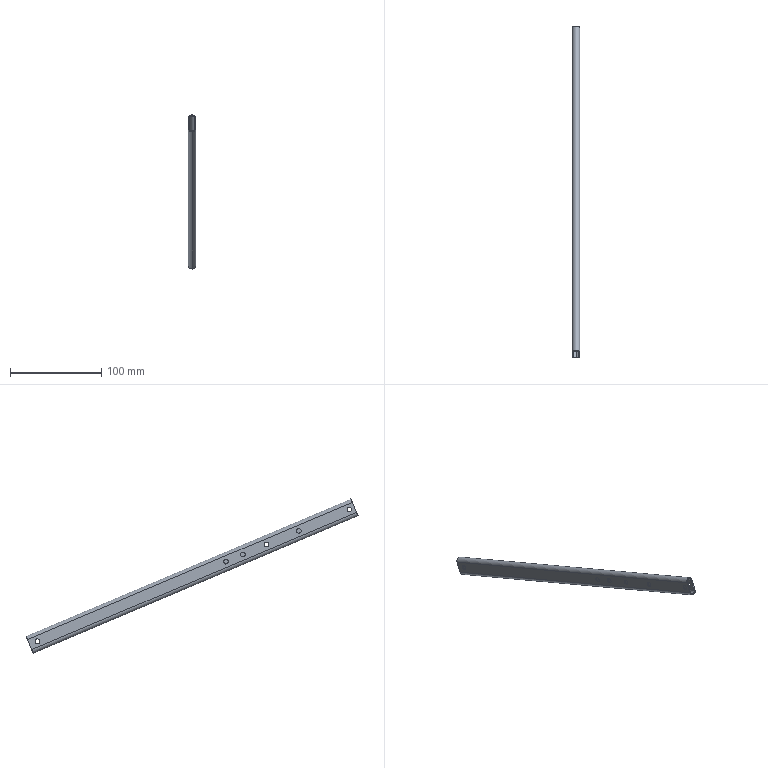Part | SolidWorks | features BaseBody 1 | 1 solid | 30 faces | box 8 x 362.948 x 168.446 mm | volume 20758 mm3 | cylinder 24 | plane 6 | commonest cylinder face diameters 5.2 x18 5.6 x3 8 x3
STEP:
#1=CARTESIAN_POINT('',(170.6,274.633,232.971));
#2=VERTEX_POINT('',#1);
#3=CARTESIAN_POINT('',(170.6,274.633,227.771));
#4=VERTEX_POINT('',#3);
#5=CARTESIAN_POINT('',(170.6,274.633,230.371));
#6=DIRECTION('',(1.,0.,0.));
#7=DIRECTION('',(0.,0.,-1.));
#8=AXIS2_PLACEMENT_3D('',#5,#6,#7);
#9=CIRCLE('',#8,2.6);
#10=EDGE_CURVE('',#2,#4,#9,.T.);
#11=ORIENTED_EDGE('',*,*,#10,.F.);
#12=CARTESIAN_POINT('',(171.8,274.633,232.971));
#13=VERTEX_POINT('',#12);
#14=CARTESIAN_POINT('',(91.8,274.633,232.971));
#15=DIRECTION('',(1.,0.,0.));
#16=VECTOR('',#15,1000.);
#17=LINE('',#14,#16);
#18=EDGE_CURVE('',#2,#13,#17,.T.);
#19=ORIENTED_EDGE('',*,*,#18,.T.);
#20=CARTESIAN_POINT('',(171.8,274.633,227.771));
#21=VERTEX_POINT('',#20);
#22=CARTESIAN_POINT('',(171.8,274.633,230.371));
#23=DIRECTION('',(-1.,0.,0.));
#24=DIRECTION('',(0.,0.,-1.));
#25=AXIS2_PLACEMENT_3D('',#22,#23,#24);
#26=CIRCLE('',#25,2.6);
#27=EDGE_CURVE('',#21,#13,#26,.T.);
#28=ORIENTED_EDGE('',*,*,#27,.F.);
#29=CARTESIAN_POINT('',(91.8,274.633,227.771));
#30=DIRECTION('',(1.,0.,0.));
#31=VECTOR('',#30,1000.);
#32=LINE('',#29,#31);
#33=EDGE_CURVE('',#4,#21,#32,.T.);
#34=ORIENTED_EDGE('',*,*,#33,.F.);
#35=EDGE_LOOP('',(#11,#19,#28,#34));
#36=FACE_OUTER_BOUND('',#35,.T.);
#37=CARTESIAN_POINT('',(91.8,274.633,230.371));
#38=DIRECTION('',(1.,0.,0.));
#39=DIRECTION('',(0.,0.,-1.));
#40=AXIS2_PLACEMENT_3D('',#37,#38,#39);
#41=CYLINDRICAL_SURFACE('',#40,2.6);
#42=ADVANCED_FACE('',(#36),#41,.F.);
#43=CARTESIAN_POINT('',(170.6,365.185,194.722));
#44=VERTEX_POINT('',#43);
#45=CARTESIAN_POINT('',(170.6,365.185,189.522));
#46=VERTEX_POINT('',#45);
#47=CARTESIAN_POINT('',(170.6,365.185,192.122));
#48=DIRECTION('',(1.,0.,0.));
#49=DIRECTION('',(0.,0.,-1.));
#50=AXIS2_PLACEMENT_3D('',#47,#48,#49);
#51=CIRCLE('',#50,2.6);
#52=EDGE_CURVE('',#44,#46,#51,.T.);
#53=ORIENTED_EDGE('',*,*,#52,.F.);
#54=CARTESIAN_POINT('',(171.8,365.185,194.722));
#55=VERTEX_POINT('',#54);
#56=CARTESIAN_POINT('',(91.8,365.185,194.722));
#57=DIRECTION('',(1.,0.,0.));
#58=VECTOR('',#57,1000.);
#59=LINE('',#56,#58);
#60=EDGE_CURVE('',#44,#55,#59,.T.);
#61=ORIENTED_EDGE('',*,*,#60,.T.);
#62=CARTESIAN_POINT('',(171.8,365.185,189.522));
#63=VERTEX_POINT('',#62);
#64=CARTESIAN_POINT('',(171.8,365.185,192.122));
#65=DIRECTION('',(-1.,0.,0.));
#66=DIRECTION('',(0.,0.,-1.));
#67=AXIS2_PLACEMENT_3D('',#64,#65,#66);
#68=CIRCLE('',#67,2.6);
#69=EDGE_CURVE('',#63,#55,#68,.T.);
#70=ORIENTED_EDGE('',*,*,#69,.F.);
#71=CARTESIAN_POINT('',(91.8,365.185,189.522));
#72=DIRECTION('',(1.,0.,0.));
#73=VECTOR('',#72,1000.);
#74=LINE('',#71,#73);
#75=EDGE_CURVE('',#46,#63,#74,.T.);
#76=ORIENTED_EDGE('',*,*,#75,.F.);
#77=EDGE_LOOP('',(#53,#61,#70,#76));
#78=FACE_OUTER_BOUND('',#77,.T.);
#79=CARTESIAN_POINT('',(91.8,365.185,192.122));
#80=DIRECTION('',(1.,0.,0.));
#81=DIRECTION('',(0.,0.,-1.));
#82=AXIS2_PLACEMENT_3D('',#79,#80,#81);
#83=CYLINDRICAL_SURFACE('',#82,2.6);
#84=ADVANCED_FACE('',(#78),#83,.F.);
#85=CARTESIAN_POINT('',(170.6,615.637,88.931));
#86=VERTEX_POINT('',#85);
#87=CARTESIAN_POINT('',(170.6,615.637,83.731));
#88=VERTEX_POINT('',#87);
#89=CARTESIAN_POINT('',(170.6,615.637,86.331));
#90=DIRECTION('',(1.,0.,0.));
#91=DIRECTION('',(0.,0.,-1.));
#92=AXIS2_PLACEMENT_3D('',#89,#90,#91);
#93=CIRCLE('',#92,2.6);
#94=EDGE_CURVE('',#86,#88,#93,.T.);
#95=ORIENTED_EDGE('',*,*,#94,.F.);
#96=CARTESIAN_POINT('',(171.8,615.637,88.931));
#97=VERTEX_POINT('',#96);
#98=CARTESIAN_POINT('',(91.8,615.637,88.931));
#99=DIRECTION('',(1.,0.,0.));
#100=VECTOR('',#99,1000.);
#101=LINE('',#98,#100);
#102=EDGE_CURVE('',#86,#97,#101,.T.);
#103=ORIENTED_EDGE('',*,*,#102,.T.);
#104=CARTESIAN_POINT('',(171.8,615.637,83.731));
#105=VERTEX_POINT('',#104);
#106=CARTESIAN_POINT('',(171.8,615.637,86.331));
#107=DIRECTION('',(-1.,0.,0.));
#108=DIRECTION('',(0.,0.,-1.));
#109=AXIS2_PLACEMENT_3D('',#106,#107,#108);
#110=CIRCLE('',#109,2.6);
#111=EDGE_CURVE('',#105,#97,#110,.T.);
#112=ORIENTED_EDGE('',*,*,#111,.F.);
#113=CARTESIAN_POINT('',(91.8,615.637,83.731));
#114=DIRECTION('',(1.,0.,0.));
#115=VECTOR('',#114,1000.);
#116=LINE('',#113,#115);
#117=EDGE_CURVE('',#88,#105,#116,.T.);
#118=ORIENTED_EDGE('',*,*,#117,.F.);
#119=EDGE_LOOP('',(#95,#103,#112,#118));
#120=FACE_OUTER_BOUND('',#119,.T.);
#121=CARTESIAN_POINT('',(91.8,615.637,86.331));
#122=DIRECTION('',(1.,0.,0.));
#123=DIRECTION('',(0.,0.,-1.));
#124=AXIS2_PLACEMENT_3D('',#121,#122,#123);
#125=CYLINDRICAL_SURFACE('',#124,2.6);
#126=ADVANCED_FACE('',(#120),#125,.F.);
#127=CARTESIAN_POINT('',(163.8,621.916,77.166));
#128=VERTEX_POINT('',#127);
#129=CARTESIAN_POINT('',(167.8,620.36,73.481));
#130=VERTEX_POINT('',#129);
#131=CARTESIAN_POINT('',(167.8,621.916,77.166));
#132=DIRECTION('',(0.,-0.9212,0.3891));
#133=DIRECTION('',(0.,-0.3891,-0.9212));
#134=AXIS2_PLACEMENT_3D('',#131,#132,#133);
#135=CIRCLE('',#134,4.);
#136=EDGE_CURVE('',#128,#130,#135,.T.);
#137=ORIENTED_EDGE('',*,*,#136,.T.);
#138=CARTESIAN_POINT('',(167.8,265.194,223.503));
#139=VERTEX_POINT('',#138);
#140=CARTESIAN_POINT('',(167.8,620.36,73.481));
#141=DIRECTION('',(0.,-0.9212,0.3891));
#142=VECTOR('',#141,1000.);
#143=LINE('',#140,#142);
#144=EDGE_CURVE('',#130,#139,#143,.T.);
#145=ORIENTED_EDGE('',*,*,#144,.T.);
#146=CARTESIAN_POINT('',(163.8,266.75,227.188));
#147=VERTEX_POINT('',#146);
#148=CARTESIAN_POINT('',(167.8,266.75,227.188));
#149=DIRECTION('',(0.,-0.9212,0.3891));
#150=DIRECTION('',(0.,-0.3891,-0.9212));
#151=AXIS2_PLACEMENT_3D('',#148,#149,#150);
#152=CIRCLE('',#151,4.);
#153=EDGE_CURVE('',#147,#139,#152,.T.);
#154=ORIENTED_EDGE('',*,*,#153,.F.);
#155=CARTESIAN_POINT('',(163.8,621.916,77.166));
#156=DIRECTION('',(0.,-0.9212,0.3891));
#157=VECTOR('',#156,1000.);
#158=LINE('',#155,#157);
#159=EDGE_CURVE('',#128,#147,#158,.T.);
#160=ORIENTED_EDGE('',*,*,#159,.F.);
#161=EDGE_LOOP('',(#137,#145,#154,#160));
#162=FACE_OUTER_BOUND('',#161,.T.);
#163=CARTESIAN_POINT('',(167.8,621.916,77.166));
#164=DIRECTION('',(0.,-0.9212,0.3891));
#165=DIRECTION('',(0.,-0.3891,-0.9212));
#166=AXIS2_PLACEMENT_3D('',#163,#164,#165);
#167=CYLINDRICAL_SURFACE('',#166,4.);
#168=ADVANCED_FACE('',(#162),#167,.T.);
#169=CARTESIAN_POINT('',(170.6,621.916,77.166));
#170=VERTEX_POINT('',#169);
#171=CARTESIAN_POINT('',(167.8,620.826,74.586));
#172=VERTEX_POINT('',#171);
#173=CARTESIAN_POINT('',(167.8,621.916,77.166));
#174=DIRECTION('',(0.,0.9212,-0.3891));
#175=DIRECTION('',(0.,-0.3891,-0.9212));
#176=AXIS2_PLACEMENT_3D('',#173,#174,#175);
#177=CIRCLE('',#176,2.8);
#178=EDGE_CURVE('',#170,#172,#177,.T.);
#179=ORIENTED_EDGE('',*,*,#178,.T.);
#180=CARTESIAN_POINT('',(167.8,265.661,224.608));
#181=VERTEX_POINT('',#180);
#182=CARTESIAN_POINT('',(167.8,620.826,74.586));
#183=DIRECTION('',(0.,-0.9212,0.3891));
#184=VECTOR('',#183,1000.);
#185=LINE('',#182,#184);
#186=EDGE_CURVE('',#172,#181,#185,.T.);
#187=ORIENTED_EDGE('',*,*,#186,.T.);
#188=CARTESIAN_POINT('',(170.6,266.75,227.188));
#189=VERTEX_POINT('',#188);
#190=CARTESIAN_POINT('',(167.8,266.75,227.188));
#191=DIRECTION('',(0.,0.9212,-0.3891));
#192=DIRECTION('',(0.,-0.3891,-0.9212));
#193=AXIS2_PLACEMENT_3D('',#190,#191,#192);
#194=CIRCLE('',#193,2.8);
#195=EDGE_CURVE('',#189,#181,#194,.T.);
#196=ORIENTED_EDGE('',*,*,#195,.F.);
#197=CARTESIAN_POINT('',(170.6,621.916,77.166));
#198=DIRECTION('',(0.,-0.9212,0.3891));
#199=VECTOR('',#198,1000.);
#200=LINE('',#197,#199);
#201=EDGE_CURVE('',#170,#189,#200,.T.);
#202=ORIENTED_EDGE('',*,*,#201,.F.);
#203=EDGE_LOOP('',(#179,#187,#196,#202));
#204=FACE_OUTER_BOUND('',#203,.T.);
#205=CARTESIAN_POINT('',(167.8,621.916,77.166));
#206=DIRECTION('',(0.,-0.9212,0.3891));
#207=DIRECTION('',(0.,-0.3891,-0.9212));
#208=AXIS2_PLACEMENT_3D('',#205,#206,#207);
#209=CYLINDRICAL_SURFACE('',#208,2.8);
#210=ADVANCED_FACE('',(#204),#209,.F.);
#211=CARTESIAN_POINT('',(165.,329.905,209.625));
#212=VERTEX_POINT('',#211);
#213=CARTESIAN_POINT('',(165.,329.905,204.425));
#214=VERTEX_POINT('',#213);
#215=CARTESIAN_POINT('',(165.,329.905,207.025));
#216=DIRECTION('',(1.,0.,0.));
#217=DIRECTION('',(0.,0.,1.));
#218=AXIS2_PLACEMENT_3D('',#215,#216,#217);
#219=CIRCLE('',#218,2.6);
#220=EDGE_CURVE('',#212,#214,#219,.T.);
#221=ORIENTED_EDGE('',*,*,#220,.T.);
#222=CARTESIAN_POINT('',(163.8,329.905,204.425));
#223=VERTEX_POINT('',#222);
#224=CARTESIAN_POINT('',(165.8,329.905,204.425));
#225=DIRECTION('',(-1.,0.,0.));
#226=VECTOR('',#225,1000.);
#227=LINE('',#224,#226);
#228=EDGE_CURVE('',#214,#223,#227,.T.);
#229=ORIENTED_EDGE('',*,*,#228,.T.);
#230=CARTESIAN_POINT('',(163.8,329.905,209.625));
#231=VERTEX_POINT('',#230);
#232=CARTESIAN_POINT('',(163.8,329.905,207.025));
#233=DIRECTION('',(1.,0.,0.));
#234=DIRECTION('',(0.,0.,1.));
#235=AXIS2_PLACEMENT_3D('',#232,#233,#234);
#236=CIRCLE('',#235,2.6);
#237=EDGE_CURVE('',#231,#223,#236,.T.);
#238=ORIENTED_EDGE('',*,*,#237,.F.);
#239=CARTESIAN_POINT('',(165.8,329.905,209.625));
#240=DIRECTION('',(-1.,0.,0.));
#241=VECTOR('',#240,1000.);
#242=LINE('',#239,#241);
#243=EDGE_CURVE('',#212,#231,#242,.T.);
#244=ORIENTED_EDGE('',*,*,#243,.F.);
#245=EDGE_LOOP('',(#221,#229,#238,#244));
#246=FACE_OUTER_BOUND('',#245,.T.);
#247=CARTESIAN_POINT('',(165.8,329.905,207.025));
#248=DIRECTION('',(-1.,0.,0.));
#249=DIRECTION('',(0.,0.,1.));
#250=AXIS2_PLACEMENT_3D('',#247,#248,#249);
#251=CYLINDRICAL_SURFACE('',#250,2.6);
#252=ADVANCED_FACE('',(#246),#251,.F.);
#253=CARTESIAN_POINT('',(163.8,274.633,232.971));
#254=VERTEX_POINT('',#253);
#255=CARTESIAN_POINT('',(163.8,274.633,227.771));
#256=VERTEX_POINT('',#255);
#257=CARTESIAN_POINT('',(163.8,274.633,230.371));
#258=DIRECTION('',(1.,0.,0.));
#259=DIRECTION('',(0.,0.,-1.));
#260=AXIS2_PLACEMENT_3D('',#257,#258,#259);
#261=CIRCLE('',#260,2.6);
#262=EDGE_CURVE('',#254,#256,#261,.T.);
#263=ORIENTED_EDGE('',*,*,#262,.F.);
#264=CARTESIAN_POINT('',(165.,274.633,232.971));
#265=VERTEX_POINT('',#264);
#266=CARTESIAN_POINT('',(91.8,274.633,232.971));
#267=DIRECTION('',(1.,0.,0.));
#268=VECTOR('',#267,1000.);
#269=LINE('',#266,#268);
#270=EDGE_CURVE('',#254,#265,#269,.T.);
#271=ORIENTED_EDGE('',*,*,#270,.T.);
#272=CARTESIAN_POINT('',(165.,274.633,227.771));
#273=VERTEX_POINT('',#272);
#274=CARTESIAN_POINT('',(165.,274.633,230.371));
#275=DIRECTION('',(1.,0.,0.));
#276=DIRECTION('',(0.,0.,-1.));
#277=AXIS2_PLACEMENT_3D('',#274,#275,#276);
#278=CIRCLE('',#277,2.6);
#279=EDGE_CURVE('',#265,#273,#278,.T.);
#280=ORIENTED_EDGE('',*,*,#279,.T.);
#281=CARTESIAN_POINT('',(91.8,274.633,227.771));
#282=DIRECTION('',(1.,0.,0.));
#283=VECTOR('',#282,1000.);
#284=LINE('',#281,#283);
#285=EDGE_CURVE('',#256,#273,#284,.T.);
#286=ORIENTED_EDGE('',*,*,#285,.F.);
#287=EDGE_LOOP('',(#263,#271,#280,#286));
#288=FACE_OUTER_BOUND('',#287,.T.);
#289=CARTESIAN_POINT('',(91.8,274.633,230.371));
#290=DIRECTION('',(1.,0.,0.));
#291=DIRECTION('',(0.,0.,-1.));
#292=AXIS2_PLACEMENT_3D('',#289,#290,#291);
#293=CYLINDRICAL_SURFACE('',#292,2.6);
#294=ADVANCED_FACE('',(#288),#293,.F.);
#295=CARTESIAN_POINT('',(163.8,365.185,194.722));
#296=VERTEX_POINT('',#295);
#297=CARTESIAN_POINT('',(163.8,365.185,189.522));
#298=VERTEX_POINT('',#297);
#299=CARTESIAN_POINT('',(163.8,365.185,192.122));
#300=DIRECTION('',(1.,0.,0.));
#301=DIRECTION('',(0.,0.,-1.));
#302=AXIS2_PLACEMENT_3D('',#299,#300,#301);
#303=CIRCLE('',#302,2.6);
#304=EDGE_CURVE('',#296,#298,#303,.T.);
#305=ORIENTED_EDGE('',*,*,#304,.F.);
#306=CARTESIAN_POINT('',(165.,365.185,194.722));
#307=VERTEX_POINT('',#306);
#308=CARTESIAN_POINT('',(91.8,365.185,194.722));
#309=DIRECTION('',(1.,0.,0.));
#310=VECTOR('',#309,1000.);
#311=LINE('',#308,#310);
#312=EDGE_CURVE('',#296,#307,#311,.T.);
#313=ORIENTED_EDGE('',*,*,#312,.T.);
#314=CARTESIAN_POINT('',(165.,365.185,189.522));
#315=VERTEX_POINT('',#314);
#316=CARTESIAN_POINT('',(165.,365.185,192.122));
#317=DIRECTION('',(1.,0.,0.));
#318=DIRECTION('',(0.,0.,-1.));
#319=AXIS2_PLACEMENT_3D('',#316,#317,#318);
#320=CIRCLE('',#319,2.6);
#321=EDGE_CURVE('',#307,#315,#320,.T.);
#322=ORIENTED_EDGE('',*,*,#321,.T.);
#323=CARTESIAN_POINT('',(91.8,365.185,189.522));
#324=DIRECTION('',(1.,0.,0.));
#325=VECTOR('',#324,1000.);
#326=LINE('',#323,#325);
#327=EDGE_CURVE('',#298,#315,#326,.T.);
#328=ORIENTED_EDGE('',*,*,#327,.F.);
#329=EDGE_LOOP('',(#305,#313,#322,#328));
#330=FACE_OUTER_BOUND('',#329,.T.);
#331=CARTESIAN_POINT('',(91.8,365.185,192.122));
#332=DIRECTION('',(1.,0.,0.));
#333=DIRECTION('',(0.,0.,-1.));
#334=AXIS2_PLACEMENT_3D('',#331,#332,#333);
#335=CYLINDRICAL_SURFACE('',#334,2.6);
#336=ADVANCED_FACE('',(#330),#335,.F.);
#337=CARTESIAN_POINT('',(163.8,615.637,88.931));
#338=VERTEX_POINT('',#337);
#339=CARTESIAN_POINT('',(163.8,615.637,83.731));
#340=VERTEX_POINT('',#339);
#341=CARTESIAN_POINT('',(163.8,615.637,86.331));
#342=DIRECTION('',(1.,0.,0.));
#343=DIRECTION('',(0.,0.,-1.));
#344=AXIS2_PLACEMENT_3D('',#341,#342,#343);
#345=CIRCLE('',#344,2.6);
#346=EDGE_CURVE('',#338,#340,#345,.T.);
#347=ORIENTED_EDGE('',*,*,#346,.F.);
#348=CARTESIAN_POINT('',(165.,615.637,88.931));
#349=VERTEX_POINT('',#348);
#350=CARTESIAN_POINT('',(91.8,615.637,88.931));
#351=DIRECTION('',(1.,0.,0.));
#352=VECTOR('',#351,1000.);
#353=LINE('',#350,#352);
#354=EDGE_CURVE('',#338,#349,#353,.T.);
#355=ORIENTED_EDGE('',*,*,#354,.T.);
#356=CARTESIAN_POINT('',(165.,615.637,83.731));
#357=VERTEX_POINT('',#356);
#358=CARTESIAN_POINT('',(165.,615.637,86.331));
#359=DIRECTION('',(1.,0.,0.));
#360=DIRECTION('',(0.,0.,-1.));
#361=AXIS2_PLACEMENT_3D('',#358,#359,#360);
#362=CIRCLE('',#361,2.6);
#363=EDGE_CURVE('',#349,#357,#362,.T.);
#364=ORIENTED_EDGE('',*,*,#363,.T.);
#365=CARTESIAN_POINT('',(91.8,615.637,83.731));
#366=DIRECTION('',(1.,0.,0.));
#367=VECTOR('',#366,1000.);
#368=LINE('',#365,#367);
#369=EDGE_CURVE('',#340,#357,#368,.T.);
#370=ORIENTED_EDGE('',*,*,#369,.F.);
#371=EDGE_LOOP('',(#347,#355,#364,#370));
#372=FACE_OUTER_BOUND('',#371,.T.);
#373=CARTESIAN_POINT('',(91.8,615.637,86.331));
#374=DIRECTION('',(1.,0.,0.));
#375=DIRECTION('',(0.,0.,-1.));
#376=AXIS2_PLACEMENT_3D('',#373,#374,#375);
#377=CYLINDRICAL_SURFACE('',#376,2.6);
#378=ADVANCED_FACE('',(#372),#377,.F.);
#379=CARTESIAN_POINT('',(165.,409.494,176.006));
#380=VERTEX_POINT('',#379);
#381=CARTESIAN_POINT('',(165.,409.494,170.806));
#382=VERTEX_POINT('',#381);
#383=CARTESIAN_POINT('',(165.,409.494,173.406));
#384=DIRECTION('',(1.,0.,0.));
#385=DIRECTION('',(0.,0.,1.));
#386=AXIS2_PLACEMENT_3D('',#383,#384,#385);
#387=CIRCLE('',#386,2.6);
#388=EDGE_CURVE('',#380,#382,#387,.T.);
#389=ORIENTED_EDGE('',*,*,#388,.T.);
#390=CARTESIAN_POINT('',(163.8,409.494,170.806));
#391=VERTEX_POINT('',#390);
#392=CARTESIAN_POINT('',(165.8,409.494,170.806));
#393=DIRECTION('',(-1.,0.,0.));
#394=VECTOR('',#393,1000.);
#395=LINE('',#392,#394);
#396=EDGE_CURVE('',#382,#391,#395,.T.);
#397=ORIENTED_EDGE('',*,*,#396,.T.);
#398=CARTESIAN_POINT('',(163.8,409.494,176.006));
#399=VERTEX_POINT('',#398);
#400=CARTESIAN_POINT('',(163.8,409.494,173.406));
#401=DIRECTION('',(1.,0.,0.));
#402=DIRECTION('',(0.,0.,1.));
#403=AXIS2_PLACEMENT_3D('',#400,#401,#402);
#404=CIRCLE('',#403,2.6);
#405=EDGE_CURVE('',#399,#391,#404,.T.);
#406=ORIENTED_EDGE('',*,*,#405,.F.);
#407=CARTESIAN_POINT('',(165.8,409.494,176.006));
#408=DIRECTION('',(-1.,0.,0.));
#409=VECTOR('',#408,1000.);
#410=LINE('',#407,#409);
#411=EDGE_CURVE('',#380,#399,#410,.T.);
#412=ORIENTED_EDGE('',*,*,#411,.F.);
#413=EDGE_LOOP('',(#389,#397,#406,#412));
#414=FACE_OUTER_BOUND('',#413,.T.);
#415=CARTESIAN_POINT('',(165.8,409.494,173.406));
#416=DIRECTION('',(-1.,0.,0.));
#417=DIRECTION('',(0.,0.,1.));
#418=AXIS2_PLACEMENT_3D('',#415,#416,#417);
#419=CYLINDRICAL_SURFACE('',#418,2.6);
#420=ADVANCED_FACE('',(#414),#419,.F.);
#421=CARTESIAN_POINT('',(165.,391.07,183.788));
#422=VERTEX_POINT('',#421);
#423=CARTESIAN_POINT('',(165.,391.07,178.588));
#424=VERTEX_POINT('',#423);
#425=CARTESIAN_POINT('',(165.,391.07,181.188));
#426=DIRECTION('',(1.,0.,0.));
#427=DIRECTION('',(0.,0.,1.));
#428=AXIS2_PLACEMENT_3D('',#425,#426,#427);
#429=CIRCLE('',#428,2.6);
#430=EDGE_CURVE('',#422,#424,#429,.T.);
#431=ORIENTED_EDGE('',*,*,#430,.T.);
#432=CARTESIAN_POINT('',(163.8,391.07,178.588));
#433=VERTEX_POINT('',#432);
#434=CARTESIAN_POINT('',(165.8,391.07,178.588));
#435=DIRECTION('',(-1.,0.,0.));
#436=VECTOR('',#435,1000.);
#437=LINE('',#434,#436);
#438=EDGE_CURVE('',#424,#433,#437,.T.);
#439=ORIENTED_EDGE('',*,*,#438,.T.);
#440=CARTESIAN_POINT('',(163.8,391.07,183.788));
#441=VERTEX_POINT('',#440);
#442=CARTESIAN_POINT('',(163.8,391.07,181.188));
#443=DIRECTION('',(1.,0.,0.));
#444=DIRECTION('',(0.,0.,1.));
#445=AXIS2_PLACEMENT_3D('',#442,#443,#444);
#446=CIRCLE('',#445,2.6);
#447=EDGE_CURVE('',#441,#433,#446,.T.);
#448=ORIENTED_EDGE('',*,*,#447,.F.);
#449=CARTESIAN_POINT('',(165.8,391.07,183.788));
#450=DIRECTION('',(-1.,0.,0.));
#451=VECTOR('',#450,1000.);
#452=LINE('',#449,#451);
#453=EDGE_CURVE('',#422,#441,#452,.T.);
#454=ORIENTED_EDGE('',*,*,#453,.F.);
#455=EDGE_LOOP('',(#431,#439,#448,#454));
#456=FACE_OUTER_BOUND('',#455,.T.);
#457=CARTESIAN_POINT('',(165.8,391.07,181.188));
#458=DIRECTION('',(-1.,0.,0.));
#459=DIRECTION('',(0.,0.,1.));
#460=AXIS2_PLACEMENT_3D('',#457,#458,#459);
#461=CYLINDRICAL_SURFACE('',#460,2.6);
#462=ADVANCED_FACE('',(#456),#461,.F.);
#463=CARTESIAN_POINT('',(163.8,271.419,238.242));
#464=VERTEX_POINT('',#463);
#465=CARTESIAN_POINT('',(171.8,271.419,238.242));
#466=VERTEX_POINT('',#465);
#467=CARTESIAN_POINT('',(167.8,271.419,238.242));
#468=DIRECTION('',(0.,0.9212,-0.3891));
#469=DIRECTION('',(0.,-0.3891,-0.9212));
#470=AXIS2_PLACEMENT_3D('',#467,#468,#469);
#471=CIRCLE('',#470,4.);
#472=EDGE_CURVE('',#464,#466,#471,.T.);
#473=ORIENTED_EDGE('',*,*,#472,.T.);
#474=CARTESIAN_POINT('',(171.8,626.585,88.22));
#475=VERTEX_POINT('',#474);
#476=CARTESIAN_POINT('',(171.8,626.585,88.22));
#477=DIRECTION('',(0.,0.9212,-0.3891));
#478=VECTOR('',#477,1000.);
#479=LINE('',#476,#478);
#480=EDGE_CURVE('',#466,#475,#479,.T.);
#481=ORIENTED_EDGE('',*,*,#480,.T.);
#482=CARTESIAN_POINT('',(163.8,626.585,88.22));
#483=VERTEX_POINT('',#482);
#484=CARTESIAN_POINT('',(167.8,626.585,88.22));
#485=DIRECTION('',(0.,-0.9212,0.3891));
#486=DIRECTION('',(0.,-0.3891,-0.9212));
#487=AXIS2_PLACEMENT_3D('',#484,#485,#486);
#488=CIRCLE('',#487,4.);
#489=EDGE_CURVE('',#475,#483,#488,.T.);
#490=ORIENTED_EDGE('',*,*,#489,.T.);
#491=CARTESIAN_POINT('',(163.8,626.585,88.22));
#492=DIRECTION('',(0.,-0.9212,0.3891));
#493=VECTOR('',#492,1000.);
#494=LINE('',#491,#493);
#495=EDGE_CURVE('',#483,#464,#494,.T.);
#496=ORIENTED_EDGE('',*,*,#495,.T.);
#497=EDGE_LOOP('',(#473,#481,#490,#496));
#498=FACE_OUTER_BOUND('',#497,.T.);
#499=CARTESIAN_POINT('',(167.8,626.585,88.22));
#500=DIRECTION('',(0.,-0.9212,0.3891));
#501=DIRECTION('',(0.,-0.3891,-0.9212));
#502=AXIS2_PLACEMENT_3D('',#499,#500,#501);
#503=CYLINDRICAL_SURFACE('',#502,4.);
#504=ADVANCED_FACE('',(#498),#503,.T.);
#505=ORIENTED_EDGE('',*,*,#27,.T.);
#506=CARTESIAN_POINT('',(171.8,274.633,230.371));
#507=DIRECTION('',(-1.,0.,0.));
#508=DIRECTION('',(0.,0.,-1.));
#509=AXIS2_PLACEMENT_3D('',#506,#507,#508);
#510=CIRCLE('',#509,2.6);
#511=EDGE_CURVE('',#13,#21,#510,.T.);
#512=ORIENTED_EDGE('',*,*,#511,.T.);
#513=EDGE_LOOP('',(#505,#512));
#514=FACE_BOUND('',#513,.T.);
#515=ORIENTED_EDGE('',*,*,#69,.T.);
#516=CARTESIAN_POINT('',(171.8,365.185,192.122));
#517=DIRECTION('',(-1.,0.,0.));
#518=DIRECTION('',(0.,0.,-1.));
#519=AXIS2_PLACEMENT_3D('',#516,#517,#518);
#520=CIRCLE('',#519,2.6);
#521=EDGE_CURVE('',#55,#63,#520,.T.);
#522=ORIENTED_EDGE('',*,*,#521,.T.);
#523=EDGE_LOOP('',(#515,#522));
#524=FACE_BOUND('',#523,.T.);
#525=ORIENTED_EDGE('',*,*,#111,.T.);
#526=CARTESIAN_POINT('',(171.8,615.637,86.331));
#527=DIRECTION('',(-1.,0.,0.));
#528=DIRECTION('',(0.,0.,-1.));
#529=AXIS2_PLACEMENT_3D('',#526,#527,#528);
#530=CIRCLE('',#529,2.6);
#531=EDGE_CURVE('',#97,#105,#530,.T.);
#532=ORIENTED_EDGE('',*,*,#531,.T.);
#533=EDGE_LOOP('',(#525,#532));
#534=FACE_BOUND('',#533,.T.);
#535=CARTESIAN_POINT('',(171.8,266.75,227.188));
#536=VERTEX_POINT('',#535);
#537=CARTESIAN_POINT('',(171.8,271.419,238.242));
#538=DIRECTION('',(0.,-0.3891,-0.9212));
#539=VECTOR('',#538,1000.);
#540=LINE('',#537,#539);
#541=EDGE_CURVE('',#466,#536,#540,.T.);
#542=ORIENTED_EDGE('',*,*,#541,.T.);
#543=CARTESIAN_POINT('',(171.8,621.916,77.166));
#544=VERTEX_POINT('',#543);
#545=CARTESIAN_POINT('',(171.8,266.75,227.188));
#546=DIRECTION('',(0.,0.9212,-0.3891));
#547=VECTOR('',#546,1000.);
#548=LINE('',#545,#547);
#549=EDGE_CURVE('',#536,#544,#548,.T.);
#550=ORIENTED_EDGE('',*,*,#549,.T.);
#551=CARTESIAN_POINT('',(171.8,621.916,77.166));
#552=DIRECTION('',(0.,0.3891,0.9212));
#553=VECTOR('',#552,1000.);
#554=LINE('',#551,#553);
#555=EDGE_CURVE('',#544,#475,#554,.T.);
#556=ORIENTED_EDGE('',*,*,#555,.T.);
#557=ORIENTED_EDGE('',*,*,#480,.F.);
#558=EDGE_LOOP('',(#542,#550,#556,#557));
#559=FACE_OUTER_BOUND('',#558,.T.);
#560=CARTESIAN_POINT('',(171.8,621.916,77.166));
#561=DIRECTION('',(1.,0.,0.));
#562=DIRECTION('',(0.,0.,-1.));
#563=AXIS2_PLACEMENT_3D('',#560,#561,#562);
#564=PLANE('',#563);
#565=ADVANCED_FACE('',(#514,#524,#534,#559),#564,.T.);
#566=CARTESIAN_POINT('',(165.,266.75,227.188));
#567=VERTEX_POINT('',#566);
#568=CARTESIAN_POINT('',(165.,271.419,238.242));
#569=VERTEX_POINT('',#568);
#570=CARTESIAN_POINT('',(165.,266.75,227.188));
#571=DIRECTION('',(0.,0.3891,0.9212));
#572=VECTOR('',#571,1000.);
#573=LINE('',#570,#572);
#574=EDGE_CURVE('',#567,#569,#573,.T.);
#575=ORIENTED_EDGE('',*,*,#574,.T.);
#576=CARTESIAN_POINT('',(170.6,271.419,238.242));
#577=VERTEX_POINT('',#576);
#578=CARTESIAN_POINT('',(167.8,271.419,238.242));
#579=DIRECTION('',(0.,0.9212,-0.3891));
#580=DIRECTION('',(0.,-0.3891,-0.9212));
#581=AXIS2_PLACEMENT_3D('',#578,#579,#580);
#582=CIRCLE('',#581,2.8);
#583=EDGE_CURVE('',#569,#577,#582,.T.);
#584=ORIENTED_EDGE('',*,*,#583,.T.);
#585=CARTESIAN_POINT('',(170.6,266.75,227.188));
#586=DIRECTION('',(0.,-0.3891,-0.9212));
#587=VECTOR('',#586,1000.);
#588=LINE('',#585,#587);
#589=EDGE_CURVE('',#577,#189,#588,.T.);
#590=ORIENTED_EDGE('',*,*,#589,.T.);
#591=ORIENTED_EDGE('',*,*,#195,.T.);
#592=CARTESIAN_POINT('',(167.8,266.75,227.188));
#593=DIRECTION('',(0.,0.9212,-0.3891));
#594=DIRECTION('',(0.,-0.3891,-0.9212));
#595=AXIS2_PLACEMENT_3D('',#592,#593,#594);
#596=CIRCLE('',#595,2.8);
#597=EDGE_CURVE('',#181,#567,#596,.T.);
#598=ORIENTED_EDGE('',*,*,#597,.T.);
#599=EDGE_LOOP('',(#575,#584,#590,#591,#598));
#600=FACE_BOUND('',#599,.T.);
#601=ORIENTED_EDGE('',*,*,#153,.T.);
#602=CARTESIAN_POINT('',(167.8,266.75,227.188));
#603=DIRECTION('',(0.,-0.9212,0.3891));
#604=DIRECTION('',(0.,-0.3891,-0.9212));
#605=AXIS2_PLACEMENT_3D('',#602,#603,#604);
#606=CIRCLE('',#605,4.);
#607=EDGE_CURVE('',#139,#536,#606,.T.);
#608=ORIENTED_EDGE('',*,*,#607,.T.);
#609=ORIENTED_EDGE('',*,*,#541,.F.);
#610=ORIENTED_EDGE('',*,*,#472,.F.);
#611=CARTESIAN_POINT('',(163.8,266.75,227.188));
#612=DIRECTION('',(0.,-0.3891,-0.9212));
#613=VECTOR('',#612,1000.);
#614=LINE('',#611,#613);
#615=EDGE_CURVE('',#464,#147,#614,.T.);
#616=ORIENTED_EDGE('',*,*,#615,.T.);
#617=EDGE_LOOP('',(#601,#608,#609,#610,#616));
#618=FACE_OUTER_BOUND('',#617,.T.);
#619=CARTESIAN_POINT('',(167.8,266.75,227.188));
#620=DIRECTION('',(0.,-0.9212,0.3891));
#621=DIRECTION('',(0.,-0.3891,-0.9212));
#622=AXIS2_PLACEMENT_3D('',#619,#620,#621);
#623=PLANE('',#622);
#624=ADVANCED_FACE('',(#600,#618),#623,.T.);
#625=ORIENTED_EDGE('',*,*,#237,.T.);
#626=CARTESIAN_POINT('',(163.8,329.905,207.025));
#627=DIRECTION('',(1.,0.,0.));
#628=DIRECTION('',(0.,0.,1.));
#629=AXIS2_PLACEMENT_3D('',#626,#627,#628);
#630=CIRCLE('',#629,2.6);
#631=EDGE_CURVE('',#223,#231,#630,.T.);
#632=ORIENTED_EDGE('',*,*,#631,.T.);
#633=EDGE_LOOP('',(#625,#632));
#634=FACE_BOUND('',#633,.T.);
#635=CARTESIAN_POINT('',(163.8,274.633,230.371));
#636=DIRECTION('',(1.,0.,0.));
#637=DIRECTION('',(0.,0.,-1.));
#638=AXIS2_PLACEMENT_3D('',#635,#636,#637);
#639=CIRCLE('',#638,2.6);
#640=EDGE_CURVE('',#256,#254,#639,.T.);
#641=ORIENTED_EDGE('',*,*,#640,.T.);
#642=ORIENTED_EDGE('',*,*,#262,.T.);
#643=EDGE_LOOP('',(#641,#642));
#644=FACE_BOUND('',#643,.T.);
#645=CARTESIAN_POINT('',(163.8,365.185,192.122));
#646=DIRECTION('',(1.,0.,0.));
#647=DIRECTION('',(0.,0.,-1.));
#648=AXIS2_PLACEMENT_3D('',#645,#646,#647);
#649=CIRCLE('',#648,2.6);
#650=EDGE_CURVE('',#298,#296,#649,.T.);
#651=ORIENTED_EDGE('',*,*,#650,.T.);
#652=ORIENTED_EDGE('',*,*,#304,.T.);
#653=EDGE_LOOP('',(#651,#652));
#654=FACE_BOUND('',#653,.T.);
#655=CARTESIAN_POINT('',(163.8,615.637,86.331));
#656=DIRECTION('',(1.,0.,0.));
#657=DIRECTION('',(0.,0.,-1.));
#658=AXIS2_PLACEMENT_3D('',#655,#656,#657);
#659=CIRCLE('',#658,2.6);
#660=EDGE_CURVE('',#340,#338,#659,.T.);
#661=ORIENTED_EDGE('',*,*,#660,.T.);
#662=ORIENTED_EDGE('',*,*,#346,.T.);
#663=EDGE_LOOP('',(#661,#662));
#664=FACE_BOUND('',#663,.T.);
#665=ORIENTED_EDGE('',*,*,#615,.F.);
#666=ORIENTED_EDGE('',*,*,#495,.F.);
#667=CARTESIAN_POINT('',(163.8,626.585,88.22));
#668=DIRECTION('',(0.,-0.3891,-0.9212));
#669=VECTOR('',#668,1000.);
#670=LINE('',#667,#669);
#671=EDGE_CURVE('',#483,#128,#670,.T.);
#672=ORIENTED_EDGE('',*,*,#671,.T.);
#673=ORIENTED_EDGE('',*,*,#159,.T.);
#674=EDGE_LOOP('',(#665,#666,#672,#673));
#675=FACE_OUTER_BOUND('',#674,.T.);
#676=ORIENTED_EDGE('',*,*,#405,.T.);
#677=CARTESIAN_POINT('',(163.8,409.494,173.406));
#678=DIRECTION('',(1.,0.,0.));
#679=DIRECTION('',(0.,0.,1.));
#680=AXIS2_PLACEMENT_3D('',#677,#678,#679);
#681=CIRCLE('',#680,2.6);
#682=EDGE_CURVE('',#391,#399,#681,.T.);
#683=ORIENTED_EDGE('',*,*,#682,.T.);
#684=EDGE_LOOP('',(#676,#683));
#685=FACE_BOUND('',#684,.T.);
#686=ORIENTED_EDGE('',*,*,#447,.T.);
#687=CARTESIAN_POINT('',(163.8,391.07,181.188));
#688=DIRECTION('',(1.,0.,0.));
#689=DIRECTION('',(0.,0.,1.));
#690=AXIS2_PLACEMENT_3D('',#687,#688,#689);
#691=CIRCLE('',#690,2.6);
#692=EDGE_CURVE('',#433,#441,#691,.T.);
#693=ORIENTED_EDGE('',*,*,#692,.T.);
#694=EDGE_LOOP('',(#686,#693));
#695=FACE_BOUND('',#694,.T.);
#696=CARTESIAN_POINT('',(163.8,621.916,77.166));
#697=DIRECTION('',(-1.,0.,0.));
#698=DIRECTION('',(0.,0.,1.));
#699=AXIS2_PLACEMENT_3D('',#696,#697,#698);
#700=PLANE('',#699);
#701=ADVANCED_FACE('',(#634,#644,#654,#664,#675,#685,#695),#700,.T.);
#702=CARTESIAN_POINT('',(170.6,626.585,88.22));
#703=VERTEX_POINT('',#702);
#704=CARTESIAN_POINT('',(170.6,621.916,77.166));
#705=DIRECTION('',(0.,-0.3891,-0.9212));
#706=VECTOR('',#705,1000.);
#707=LINE('',#704,#706);
#708=EDGE_CURVE('',#703,#170,#707,.T.);
#709=ORIENTED_EDGE('',*,*,#708,.F.);
#710=CARTESIAN_POINT('',(165.,626.585,88.22));
#711=VERTEX_POINT('',#710);
#712=CARTESIAN_POINT('',(167.8,626.585,88.22));
#713=DIRECTION('',(0.,0.9212,-0.3891));
#714=DIRECTION('',(0.,-0.3891,-0.9212));
#715=AXIS2_PLACEMENT_3D('',#712,#713,#714);
#716=CIRCLE('',#715,2.8);
#717=EDGE_CURVE('',#711,#703,#716,.T.);
#718=ORIENTED_EDGE('',*,*,#717,.F.);
#719=CARTESIAN_POINT('',(165.,621.916,77.166));
#720=VERTEX_POINT('',#719);
#721=CARTESIAN_POINT('',(165.,621.916,77.166));
#722=DIRECTION('',(0.,0.3891,0.9212));
#723=VECTOR('',#722,1000.);
#724=LINE('',#721,#723);
#725=EDGE_CURVE('',#720,#711,#724,.T.);
#726=ORIENTED_EDGE('',*,*,#725,.F.);
#727=CARTESIAN_POINT('',(167.8,621.916,77.166));
#728=DIRECTION('',(0.,0.9212,-0.3891));
#729=DIRECTION('',(0.,-0.3891,-0.9212));
#730=AXIS2_PLACEMENT_3D('',#727,#728,#729);
#731=CIRCLE('',#730,2.8);
#732=EDGE_CURVE('',#172,#720,#731,.T.);
#733=ORIENTED_EDGE('',*,*,#732,.F.);
#734=ORIENTED_EDGE('',*,*,#178,.F.);
#735=EDGE_LOOP('',(#709,#718,#726,#733,#734));
#736=FACE_BOUND('',#735,.T.);
#737=ORIENTED_EDGE('',*,*,#489,.F.);
#738=ORIENTED_EDGE('',*,*,#555,.F.);
#739=CARTESIAN_POINT('',(167.8,621.916,77.166));
#740=DIRECTION('',(0.,-0.9212,0.3891));
#741=DIRECTION('',(0.,-0.3891,-0.9212));
#742=AXIS2_PLACEMENT_3D('',#739,#740,#741);
#743=CIRCLE('',#742,4.);
#744=EDGE_CURVE('',#130,#544,#743,.T.);
#745=ORIENTED_EDGE('',*,*,#744,.F.);
#746=ORIENTED_EDGE('',*,*,#136,.F.);
#747=ORIENTED_EDGE('',*,*,#671,.F.);
#748=EDGE_LOOP('',(#737,#738,#745,#746,#747));
#749=FACE_OUTER_BOUND('',#748,.T.);
#750=CARTESIAN_POINT('',(167.8,621.916,77.166));
#751=DIRECTION('',(0.,-0.9212,0.3891));
#752=DIRECTION('',(0.,-0.3891,-0.9212));
#753=AXIS2_PLACEMENT_3D('',#750,#751,#752);
#754=PLANE('',#753);
#755=ADVANCED_FACE('',(#736,#749),#754,.F.);
#756=ORIENTED_EDGE('',*,*,#18,.F.);
#757=CARTESIAN_POINT('',(170.6,274.633,230.371));
#758=DIRECTION('',(1.,0.,0.));
#759=DIRECTION('',(0.,0.,-1.));
#760=AXIS2_PLACEMENT_3D('',#757,#758,#759);
#761=CIRCLE('',#760,2.6);
#762=EDGE_CURVE('',#4,#2,#761,.T.);
#763=ORIENTED_EDGE('',*,*,#762,.F.);
#764=ORIENTED_EDGE('',*,*,#33,.T.);
#765=ORIENTED_EDGE('',*,*,#511,.F.);
#766=EDGE_LOOP('',(#756,#763,#764,#765));
#767=FACE_OUTER_BOUND('',#766,.T.);
#768=CARTESIAN_POINT('',(91.8,274.633,230.371));
#769=DIRECTION('',(1.,0.,0.));
#770=DIRECTION('',(0.,0.,-1.));
#771=AXIS2_PLACEMENT_3D('',#768,#769,#770);
#772=CYLINDRICAL_SURFACE('',#771,2.6);
#773=ADVANCED_FACE('',(#767),#772,.F.);
#774=ORIENTED_EDGE('',*,*,#60,.F.);
#775=CARTESIAN_POINT('',(170.6,365.185,192.122));
#776=DIRECTION('',(1.,0.,0.));
#777=DIRECTION('',(0.,0.,-1.));
#778=AXIS2_PLACEMENT_3D('',#775,#776,#777);
#779=CIRCLE('',#778,2.6);
#780=EDGE_CURVE('',#46,#44,#779,.T.);
#781=ORIENTED_EDGE('',*,*,#780,.F.);
#782=ORIENTED_EDGE('',*,*,#75,.T.);
#783=ORIENTED_EDGE('',*,*,#521,.F.);
#784=EDGE_LOOP('',(#774,#781,#782,#783));
#785=FACE_OUTER_BOUND('',#784,.T.);
#786=CARTESIAN_POINT('',(91.8,365.185,192.122));
#787=DIRECTION('',(1.,0.,0.));
#788=DIRECTION('',(0.,0.,-1.));
#789=AXIS2_PLACEMENT_3D('',#786,#787,#788);
#790=CYLINDRICAL_SURFACE('',#789,2.6);
#791=ADVANCED_FACE('',(#785),#790,.F.);
#792=ORIENTED_EDGE('',*,*,#102,.F.);
#793=CARTESIAN_POINT('',(170.6,615.637,86.331));
#794=DIRECTION('',(1.,0.,0.));
#795=DIRECTION('',(0.,0.,-1.));
#796=AXIS2_PLACEMENT_3D('',#793,#794,#795);
#797=CIRCLE('',#796,2.6);
#798=EDGE_CURVE('',#88,#86,#797,.T.);
#799=ORIENTED_EDGE('',*,*,#798,.F.);
#800=ORIENTED_EDGE('',*,*,#117,.T.);
#801=ORIENTED_EDGE('',*,*,#531,.F.);
#802=EDGE_LOOP('',(#792,#799,#800,#801));
#803=FACE_OUTER_BOUND('',#802,.T.);
#804=CARTESIAN_POINT('',(91.8,615.637,86.331));
#805=DIRECTION('',(1.,0.,0.));
#806=DIRECTION('',(0.,0.,-1.));
#807=AXIS2_PLACEMENT_3D('',#804,#805,#806);
#808=CYLINDRICAL_SURFACE('',#807,2.6);
#809=ADVANCED_FACE('',(#803),#808,.F.);
#810=ORIENTED_EDGE('',*,*,#144,.F.);
#811=ORIENTED_EDGE('',*,*,#744,.T.);
#812=ORIENTED_EDGE('',*,*,#549,.F.);
#813=ORIENTED_EDGE('',*,*,#607,.F.);
#814=EDGE_LOOP('',(#810,#811,#812,#813));
#815=FACE_OUTER_BOUND('',#814,.T.);
#816=CARTESIAN_POINT('',(167.8,621.916,77.166));
#817=DIRECTION('',(0.,-0.9212,0.3891));
#818=DIRECTION('',(0.,-0.3891,-0.9212));
#819=AXIS2_PLACEMENT_3D('',#816,#817,#818);
#820=CYLINDRICAL_SURFACE('',#819,4.);
#821=ADVANCED_FACE('',(#815),#820,.T.);
#822=ORIENTED_EDGE('',*,*,#717,.T.);
#823=CARTESIAN_POINT('',(170.6,626.585,88.22));
#824=DIRECTION('',(0.,0.9212,-0.3891));
#825=VECTOR('',#824,1000.);
#826=LINE('',#823,#825);
#827=EDGE_CURVE('',#577,#703,#826,.T.);
#828=ORIENTED_EDGE('',*,*,#827,.F.);
#829=ORIENTED_EDGE('',*,*,#583,.F.);
#830=CARTESIAN_POINT('',(165.,626.585,88.22));
#831=DIRECTION('',(0.,-0.9212,0.3891));
#832=VECTOR('',#831,1000.);
#833=LINE('',#830,#832);
#834=EDGE_CURVE('',#711,#569,#833,.T.);
#835=ORIENTED_EDGE('',*,*,#834,.F.);
#836=EDGE_LOOP('',(#822,#828,#829,#835));
#837=FACE_OUTER_BOUND('',#836,.T.);
#838=CARTESIAN_POINT('',(167.8,626.585,88.22));
#839=DIRECTION('',(0.,-0.9212,0.3891));
#840=DIRECTION('',(0.,-0.3891,-0.9212));
#841=AXIS2_PLACEMENT_3D('',#838,#839,#840);
#842=CYLINDRICAL_SURFACE('',#841,2.8);
#843=ADVANCED_FACE('',(#837),#842,.F.);
#844=ORIENTED_EDGE('',*,*,#220,.F.);
#845=CARTESIAN_POINT('',(165.,329.905,207.025));
#846=DIRECTION('',(1.,0.,0.));
#847=DIRECTION('',(0.,0.,1.));
#848=AXIS2_PLACEMENT_3D('',#845,#846,#847);
#849=CIRCLE('',#848,2.6);
#850=EDGE_CURVE('',#214,#212,#849,.T.);
#851=ORIENTED_EDGE('',*,*,#850,.F.);
#852=EDGE_LOOP('',(#844,#851));
#853=FACE_BOUND('',#852,.T.);
#854=CARTESIAN_POINT('',(165.,274.633,230.371));
#855=DIRECTION('',(1.,0.,0.));
#856=DIRECTION('',(0.,0.,-1.));
#857=AXIS2_PLACEMENT_3D('',#854,#855,#856);
#858=CIRCLE('',#857,2.6);
#859=EDGE_CURVE('',#273,#265,#858,.T.);
#860=ORIENTED_EDGE('',*,*,#859,.F.);
#861=ORIENTED_EDGE('',*,*,#279,.F.);
#862=EDGE_LOOP('',(#860,#861));
#863=FACE_BOUND('',#862,.T.);
#864=CARTESIAN_POINT('',(165.,365.185,192.122));
#865=DIRECTION('',(1.,0.,0.));
#866=DIRECTION('',(0.,0.,-1.));
#867=AXIS2_PLACEMENT_3D('',#864,#865,#866);
#868=CIRCLE('',#867,2.6);
#869=EDGE_CURVE('',#315,#307,#868,.T.);
#870=ORIENTED_EDGE('',*,*,#869,.F.);
#871=ORIENTED_EDGE('',*,*,#321,.F.);
#872=EDGE_LOOP('',(#870,#871));
#873=FACE_BOUND('',#872,.T.);
#874=CARTESIAN_POINT('',(165.,615.637,86.331));
#875=DIRECTION('',(1.,0.,0.));
#876=DIRECTION('',(0.,0.,-1.));
#877=AXIS2_PLACEMENT_3D('',#874,#875,#876);
#878=CIRCLE('',#877,2.6);
#879=EDGE_CURVE('',#357,#349,#878,.T.);
#880=ORIENTED_EDGE('',*,*,#879,.F.);
#881=ORIENTED_EDGE('',*,*,#363,.F.);
#882=EDGE_LOOP('',(#880,#881));
#883=FACE_BOUND('',#882,.T.);
#884=ORIENTED_EDGE('',*,*,#725,.T.);
#885=ORIENTED_EDGE('',*,*,#834,.T.);
#886=ORIENTED_EDGE('',*,*,#574,.F.);
#887=CARTESIAN_POINT('',(165.,621.916,77.166));
#888=DIRECTION('',(0.,-0.9212,0.3891));
#889=VECTOR('',#888,1000.);
#890=LINE('',#887,#889);
#891=EDGE_CURVE('',#720,#567,#890,.T.);
#892=ORIENTED_EDGE('',*,*,#891,.F.);
#893=EDGE_LOOP('',(#884,#885,#886,#892));
#894=FACE_OUTER_BOUND('',#893,.T.);
#895=ORIENTED_EDGE('',*,*,#388,.F.);
#896=CARTESIAN_POINT('',(165.,409.494,173.406));
#897=DIRECTION('',(1.,0.,0.));
#898=DIRECTION('',(0.,0.,1.));
#899=AXIS2_PLACEMENT_3D('',#896,#897,#898);
#900=CIRCLE('',#899,2.6);
#901=EDGE_CURVE('',#382,#380,#900,.T.);
#902=ORIENTED_EDGE('',*,*,#901,.F.);
#903=EDGE_LOOP('',(#895,#902));
#904=FACE_BOUND('',#903,.T.);
#905=ORIENTED_EDGE('',*,*,#430,.F.);
#906=CARTESIAN_POINT('',(165.,391.07,181.188));
#907=DIRECTION('',(1.,0.,0.));
#908=DIRECTION('',(0.,0.,1.));
#909=AXIS2_PLACEMENT_3D('',#906,#907,#908);
#910=CIRCLE('',#909,2.6);
#911=EDGE_CURVE('',#424,#422,#910,.T.);
#912=ORIENTED_EDGE('',*,*,#911,.F.);
#913=EDGE_LOOP('',(#905,#912));
#914=FACE_BOUND('',#913,.T.);
#915=CARTESIAN_POINT('',(165.,621.916,77.166));
#916=DIRECTION('',(-1.,0.,0.));
#917=DIRECTION('',(0.,0.,1.));
#918=AXIS2_PLACEMENT_3D('',#915,#916,#917);
#919=PLANE('',#918);
#920=ADVANCED_FACE('',(#853,#863,#873,#883,#894,#904,#914),#919,.F.);
#921=ORIENTED_EDGE('',*,*,#186,.F.);
#922=ORIENTED_EDGE('',*,*,#732,.T.);
#923=ORIENTED_EDGE('',*,*,#891,.T.);
#924=ORIENTED_EDGE('',*,*,#597,.F.);
#925=EDGE_LOOP('',(#921,#922,#923,#924));
#926=FACE_OUTER_BOUND('',#925,.T.);
#927=CARTESIAN_POINT('',(167.8,621.916,77.166));
#928=DIRECTION('',(0.,-0.9212,0.3891));
#929=DIRECTION('',(0.,-0.3891,-0.9212));
#930=AXIS2_PLACEMENT_3D('',#927,#928,#929);
#931=CYLINDRICAL_SURFACE('',#930,2.8);
#932=ADVANCED_FACE('',(#926),#931,.F.);
#933=ORIENTED_EDGE('',*,*,#762,.T.);
#934=ORIENTED_EDGE('',*,*,#10,.T.);
#935=EDGE_LOOP('',(#933,#934));
#936=FACE_BOUND('',#935,.T.);
#937=ORIENTED_EDGE('',*,*,#780,.T.);
#938=ORIENTED_EDGE('',*,*,#52,.T.);
#939=EDGE_LOOP('',(#937,#938));
#940=FACE_BOUND('',#939,.T.);
#941=ORIENTED_EDGE('',*,*,#798,.T.);
#942=ORIENTED_EDGE('',*,*,#94,.T.);
#943=EDGE_LOOP('',(#941,#942));
#944=FACE_BOUND('',#943,.T.);
#945=ORIENTED_EDGE('',*,*,#708,.T.);
#946=ORIENTED_EDGE('',*,*,#201,.T.);
#947=ORIENTED_EDGE('',*,*,#589,.F.);
#948=ORIENTED_EDGE('',*,*,#827,.T.);
#949=EDGE_LOOP('',(#945,#946,#947,#948));
#950=FACE_OUTER_BOUND('',#949,.T.);
#951=CARTESIAN_POINT('',(170.6,621.916,77.166));
#952=DIRECTION('',(1.,0.,0.));
#953=DIRECTION('',(0.,0.,-1.));
#954=AXIS2_PLACEMENT_3D('',#951,#952,#953);
#955=PLANE('',#954);
#956=ADVANCED_FACE('',(#936,#940,#944,#950),#955,.F.);
#957=ORIENTED_EDGE('',*,*,#228,.F.);
#958=ORIENTED_EDGE('',*,*,#850,.T.);
#959=ORIENTED_EDGE('',*,*,#243,.T.);
#960=ORIENTED_EDGE('',*,*,#631,.F.);
#961=EDGE_LOOP('',(#957,#958,#959,#960));
#962=FACE_OUTER_BOUND('',#961,.T.);
#963=CARTESIAN_POINT('',(165.8,329.905,207.025));
#964=DIRECTION('',(-1.,0.,0.));
#965=DIRECTION('',(0.,0.,1.));
#966=AXIS2_PLACEMENT_3D('',#963,#964,#965);
#967=CYLINDRICAL_SURFACE('',#966,2.6);
#968=ADVANCED_FACE('',(#962),#967,.F.);
#969=ORIENTED_EDGE('',*,*,#270,.F.);
#970=ORIENTED_EDGE('',*,*,#640,.F.);
#971=ORIENTED_EDGE('',*,*,#285,.T.);
#972=ORIENTED_EDGE('',*,*,#859,.T.);
#973=EDGE_LOOP('',(#969,#970,#971,#972));
#974=FACE_OUTER_BOUND('',#973,.T.);
#975=CARTESIAN_POINT('',(91.8,274.633,230.371));
#976=DIRECTION('',(1.,0.,0.));
#977=DIRECTION('',(0.,0.,-1.));
#978=AXIS2_PLACEMENT_3D('',#975,#976,#977);
#979=CYLINDRICAL_SURFACE('',#978,2.6);
#980=ADVANCED_FACE('',(#974),#979,.F.);
#981=ORIENTED_EDGE('',*,*,#312,.F.);
#982=ORIENTED_EDGE('',*,*,#650,.F.);
#983=ORIENTED_EDGE('',*,*,#327,.T.);
#984=ORIENTED_EDGE('',*,*,#869,.T.);
#985=EDGE_LOOP('',(#981,#982,#983,#984));
#986=FACE_OUTER_BOUND('',#985,.T.);
#987=CARTESIAN_POINT('',(91.8,365.185,192.122));
#988=DIRECTION('',(1.,0.,0.));
#989=DIRECTION('',(0.,0.,-1.));
#990=AXIS2_PLACEMENT_3D('',#987,#988,#989);
#991=CYLINDRICAL_SURFACE('',#990,2.6);
#992=ADVANCED_FACE('',(#986),#991,.F.);
#993=ORIENTED_EDGE('',*,*,#354,.F.);
#994=ORIENTED_EDGE('',*,*,#660,.F.);
#995=ORIENTED_EDGE('',*,*,#369,.T.);
#996=ORIENTED_EDGE('',*,*,#879,.T.);
#997=EDGE_LOOP('',(#993,#994,#995,#996));
#998=FACE_OUTER_BOUND('',#997,.T.);
#999=CARTESIAN_POINT('',(91.8,615.637,86.331));
#1000=DIRECTION('',(1.,0.,0.));
#1001=DIRECTION('',(0.,0.,-1.));
#1002=AXIS2_PLACEMENT_3D('',#999,#1000,#1001);
#1003=CYLINDRICAL_SURFACE('',#1002,2.6);
#1004=ADVANCED_FACE('',(#998),#1003,.F.);
#1005=ORIENTED_EDGE('',*,*,#396,.F.);
#1006=ORIENTED_EDGE('',*,*,#901,.T.);
#1007=ORIENTED_EDGE('',*,*,#411,.T.);
#1008=ORIENTED_EDGE('',*,*,#682,.F.);
#1009=EDGE_LOOP('',(#1005,#1006,#1007,#1008));
#1010=FACE_OUTER_BOUND('',#1009,.T.);
#1011=CARTESIAN_POINT('',(165.8,409.494,173.406));
#1012=DIRECTION('',(-1.,0.,0.));
#1013=DIRECTION('',(0.,0.,1.));
#1014=AXIS2_PLACEMENT_3D('',#1011,#1012,#1013);
#1015=CYLINDRICAL_SURFACE('',#1014,2.6);
#1016=ADVANCED_FACE('',(#1010),#1015,.F.);
#1017=ORIENTED_EDGE('',*,*,#438,.F.);
#1018=ORIENTED_EDGE('',*,*,#911,.T.);
#1019=ORIENTED_EDGE('',*,*,#453,.T.);
#1020=ORIENTED_EDGE('',*,*,#692,.F.);
#1021=EDGE_LOOP('',(#1017,#1018,#1019,#1020));
#1022=FACE_OUTER_BOUND('',#1021,.T.);
#1023=CARTESIAN_POINT('',(165.8,391.07,181.188));
#1024=DIRECTION('',(-1.,0.,0.));
#1025=DIRECTION('',(0.,0.,1.));
#1026=AXIS2_PLACEMENT_3D('',#1023,#1024,#1025);
#1027=CYLINDRICAL_SURFACE('',#1026,2.6);
#1028=ADVANCED_FACE('',(#1022),#1027,.F.);
#1029=CLOSED_SHELL('',(#42,#84,#126,#168,#210,#252,#294,#336,#378,#420,#462,#504,#565,#624,#701,#755,#773,#791,#809,#821,#843,#920,#932,#956,#968,#980,#992,#1004,#1016,#1028));
#1030=MANIFOLD_SOLID_BREP('',#1029);
#1031=CARTESIAN_POINT('',(0.,0.,0.));
#1032=DIRECTION('',(0.,0.,1.));
#1033=DIRECTION('',(1.,0.,0.));
#1034=AXIS2_PLACEMENT_3D('',#1031,#1032,#1033);
#1035=(LENGTH_UNIT()NAMED_UNIT(*)SI_UNIT(.MILLI.,.METRE.));
#1036=UNCERTAINTY_MEASURE_WITH_UNIT(LENGTH_MEASURE(0.00001),#1035,'','');
#1037=(NAMED_UNIT(*)PLANE_ANGLE_UNIT()SI_UNIT($,.RADIAN.));
#1038=(NAMED_UNIT(*)SI_UNIT($,.STERADIAN.)SOLID_ANGLE_UNIT());
#1039=(GEOMETRIC_REPRESENTATION_CONTEXT(3)GLOBAL_UNCERTAINTY_ASSIGNED_CONTEXT((#1036))GLOBAL_UNIT_ASSIGNED_CONTEXT((#1035,#1037,#1038))REPRESENTATION_CONTEXT('',''));
#1040=ADVANCED_BREP_SHAPE_REPRESENTATION('',(#1030,#1034),#1039);